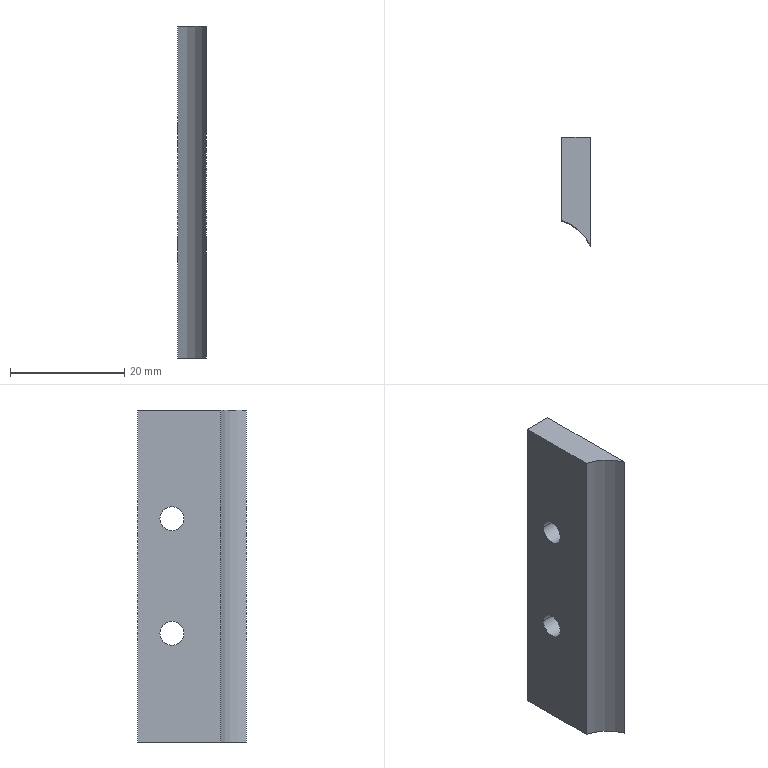Part | SolidWorks | features Extrusion 1, ICE 1 | 1 solid | 10 faces | box 5 x 19 x 58 mm | volume 4522 mm3 | cylinder 5 | plane 5 | commonest cylinder face diameters 4.2 x4 15.6 x1
STEP:
#1=CARTESIAN_POINT('',(2.222,2.186,19.));
#2=VERTEX_POINT('',#1);
#3=CARTESIAN_POINT('',(2.222,-2.014,19.));
#4=VERTEX_POINT('',#3);
#5=CARTESIAN_POINT('',(2.222,0.08586,19.));
#6=DIRECTION('',(-1.,0.,0.));
#7=DIRECTION('',(0.,-1.,0.));
#8=AXIS2_PLACEMENT_3D('',#5,#6,#7);
#9=CIRCLE('',#8,2.1);
#10=EDGE_CURVE('',#2,#4,#9,.T.);
#11=ORIENTED_EDGE('',*,*,#10,.F.);
#12=CARTESIAN_POINT('',(-2.778,2.186,19.));
#13=VERTEX_POINT('',#12);
#14=CARTESIAN_POINT('',(2.222,2.186,19.));
#15=DIRECTION('',(-1.,0.,0.));
#16=VECTOR('',#15,1000.);
#17=LINE('',#14,#16);
#18=EDGE_CURVE('',#2,#13,#17,.T.);
#19=ORIENTED_EDGE('',*,*,#18,.T.);
#20=CARTESIAN_POINT('',(-2.778,-2.014,19.));
#21=VERTEX_POINT('',#20);
#22=CARTESIAN_POINT('',(-2.778,0.08586,19.));
#23=DIRECTION('',(-1.,0.,0.));
#24=DIRECTION('',(0.,-1.,0.));
#25=AXIS2_PLACEMENT_3D('',#22,#23,#24);
#26=CIRCLE('',#25,2.1);
#27=EDGE_CURVE('',#13,#21,#26,.T.);
#28=ORIENTED_EDGE('',*,*,#27,.T.);
#29=CARTESIAN_POINT('',(2.222,-2.014,19.));
#30=DIRECTION('',(-1.,0.,0.));
#31=VECTOR('',#30,1000.);
#32=LINE('',#29,#31);
#33=EDGE_CURVE('',#4,#21,#32,.T.);
#34=ORIENTED_EDGE('',*,*,#33,.F.);
#35=EDGE_LOOP('',(#11,#19,#28,#34));
#36=FACE_OUTER_BOUND('',#35,.T.);
#37=CARTESIAN_POINT('',(2.222,0.08586,19.));
#38=DIRECTION('',(-1.,0.,0.));
#39=DIRECTION('',(0.,-1.,0.));
#40=AXIS2_PLACEMENT_3D('',#37,#38,#39);
#41=CYLINDRICAL_SURFACE('',#40,2.1);
#42=ADVANCED_FACE('',(#36),#41,.F.);
#43=CARTESIAN_POINT('',(2.222,2.186,39.));
#44=VERTEX_POINT('',#43);
#45=CARTESIAN_POINT('',(2.222,-2.014,39.));
#46=VERTEX_POINT('',#45);
#47=CARTESIAN_POINT('',(2.222,0.08586,39.));
#48=DIRECTION('',(-1.,0.,0.));
#49=DIRECTION('',(0.,-1.,0.));
#50=AXIS2_PLACEMENT_3D('',#47,#48,#49);
#51=CIRCLE('',#50,2.1);
#52=EDGE_CURVE('',#44,#46,#51,.T.);
#53=ORIENTED_EDGE('',*,*,#52,.F.);
#54=CARTESIAN_POINT('',(-2.778,2.186,39.));
#55=VERTEX_POINT('',#54);
#56=CARTESIAN_POINT('',(2.222,2.186,39.));
#57=DIRECTION('',(-1.,0.,0.));
#58=VECTOR('',#57,1000.);
#59=LINE('',#56,#58);
#60=EDGE_CURVE('',#44,#55,#59,.T.);
#61=ORIENTED_EDGE('',*,*,#60,.T.);
#62=CARTESIAN_POINT('',(-2.778,-2.014,39.));
#63=VERTEX_POINT('',#62);
#64=CARTESIAN_POINT('',(-2.778,0.08586,39.));
#65=DIRECTION('',(-1.,0.,0.));
#66=DIRECTION('',(0.,-1.,0.));
#67=AXIS2_PLACEMENT_3D('',#64,#65,#66);
#68=CIRCLE('',#67,2.1);
#69=EDGE_CURVE('',#55,#63,#68,.T.);
#70=ORIENTED_EDGE('',*,*,#69,.T.);
#71=CARTESIAN_POINT('',(2.222,-2.014,39.));
#72=DIRECTION('',(-1.,0.,0.));
#73=VECTOR('',#72,1000.);
#74=LINE('',#71,#73);
#75=EDGE_CURVE('',#46,#63,#74,.T.);
#76=ORIENTED_EDGE('',*,*,#75,.F.);
#77=EDGE_LOOP('',(#53,#61,#70,#76));
#78=FACE_OUTER_BOUND('',#77,.T.);
#79=CARTESIAN_POINT('',(2.222,0.08586,39.));
#80=DIRECTION('',(-1.,0.,0.));
#81=DIRECTION('',(0.,-1.,0.));
#82=AXIS2_PLACEMENT_3D('',#79,#80,#81);
#83=CYLINDRICAL_SURFACE('',#82,2.1);
#84=ADVANCED_FACE('',(#78),#83,.F.);
#85=CARTESIAN_POINT('',(-2.778,0.08586,19.));
#86=DIRECTION('',(-1.,0.,0.));
#87=DIRECTION('',(0.,-1.,0.));
#88=AXIS2_PLACEMENT_3D('',#85,#86,#87);
#89=CIRCLE('',#88,2.1);
#90=EDGE_CURVE('',#21,#13,#89,.T.);
#91=ORIENTED_EDGE('',*,*,#90,.F.);
#92=ORIENTED_EDGE('',*,*,#27,.F.);
#93=EDGE_LOOP('',(#91,#92));
#94=FACE_BOUND('',#93,.T.);
#95=CARTESIAN_POINT('',(-2.778,0.08586,39.));
#96=DIRECTION('',(-1.,0.,0.));
#97=DIRECTION('',(0.,-1.,0.));
#98=AXIS2_PLACEMENT_3D('',#95,#96,#97);
#99=CIRCLE('',#98,2.1);
#100=EDGE_CURVE('',#63,#55,#99,.T.);
#101=ORIENTED_EDGE('',*,*,#100,.F.);
#102=ORIENTED_EDGE('',*,*,#69,.F.);
#103=EDGE_LOOP('',(#101,#102));
#104=FACE_BOUND('',#103,.T.);
#105=CARTESIAN_POINT('',(-2.778,6.086,0.));
#106=VERTEX_POINT('',#105);
#107=CARTESIAN_POINT('',(-2.778,-8.431,0.));
#108=VERTEX_POINT('',#107);
#109=CARTESIAN_POINT('',(-2.778,6.086,0.));
#110=DIRECTION('',(0.,-1.,0.));
#111=VECTOR('',#110,1000.);
#112=LINE('',#109,#111);
#113=EDGE_CURVE('',#106,#108,#112,.T.);
#114=ORIENTED_EDGE('',*,*,#113,.T.);
#115=CARTESIAN_POINT('',(-2.778,-8.431,58.));
#116=VERTEX_POINT('',#115);
#117=CARTESIAN_POINT('',(-2.778,-8.431,58.));
#118=DIRECTION('',(0.,0.,-1.));
#119=VECTOR('',#118,1000.);
#120=LINE('',#117,#119);
#121=EDGE_CURVE('',#116,#108,#120,.T.);
#122=ORIENTED_EDGE('',*,*,#121,.F.);
#123=CARTESIAN_POINT('',(-2.778,6.086,58.));
#124=VERTEX_POINT('',#123);
#125=CARTESIAN_POINT('',(-2.778,6.086,58.));
#126=DIRECTION('',(0.,-1.,0.));
#127=VECTOR('',#126,1000.);
#128=LINE('',#125,#127);
#129=EDGE_CURVE('',#124,#116,#128,.T.);
#130=ORIENTED_EDGE('',*,*,#129,.F.);
#131=CARTESIAN_POINT('',(-2.778,6.086,58.));
#132=DIRECTION('',(0.,0.,-1.));
#133=VECTOR('',#132,1000.);
#134=LINE('',#131,#133);
#135=EDGE_CURVE('',#124,#106,#134,.T.);
#136=ORIENTED_EDGE('',*,*,#135,.T.);
#137=EDGE_LOOP('',(#114,#122,#130,#136));
#138=FACE_OUTER_BOUND('',#137,.T.);
#139=CARTESIAN_POINT('',(-2.778,6.086,58.));
#140=DIRECTION('',(1.,0.,0.));
#141=DIRECTION('',(0.,1.,0.));
#142=AXIS2_PLACEMENT_3D('',#139,#140,#141);
#143=PLANE('',#142);
#144=ADVANCED_FACE('',(#94,#104,#138),#143,.F.);
#145=CARTESIAN_POINT('',(2.222,-12.914,0.));
#146=VERTEX_POINT('',#145);
#147=CARTESIAN_POINT('',(-4.978,-15.914,0.));
#148=DIRECTION('',(0.,0.,-1.));
#149=DIRECTION('',(1.,0.,0.));
#150=AXIS2_PLACEMENT_3D('',#147,#148,#149);
#151=CIRCLE('',#150,7.8);
#152=EDGE_CURVE('',#108,#146,#151,.T.);
#153=ORIENTED_EDGE('',*,*,#152,.T.);
#154=CARTESIAN_POINT('',(2.222,-12.914,58.));
#155=VERTEX_POINT('',#154);
#156=CARTESIAN_POINT('',(2.222,-12.914,58.));
#157=DIRECTION('',(0.,0.,-1.));
#158=VECTOR('',#157,1000.);
#159=LINE('',#156,#158);
#160=EDGE_CURVE('',#155,#146,#159,.T.);
#161=ORIENTED_EDGE('',*,*,#160,.F.);
#162=CARTESIAN_POINT('',(-4.978,-15.914,58.));
#163=DIRECTION('',(0.,0.,-1.));
#164=DIRECTION('',(1.,0.,0.));
#165=AXIS2_PLACEMENT_3D('',#162,#163,#164);
#166=CIRCLE('',#165,7.8);
#167=EDGE_CURVE('',#116,#155,#166,.T.);
#168=ORIENTED_EDGE('',*,*,#167,.F.);
#169=ORIENTED_EDGE('',*,*,#121,.T.);
#170=EDGE_LOOP('',(#153,#161,#168,#169));
#171=FACE_OUTER_BOUND('',#170,.T.);
#172=CARTESIAN_POINT('',(-4.978,-15.914,58.));
#173=DIRECTION('',(0.,0.,-1.));
#174=DIRECTION('',(-1.,0.,0.));
#175=AXIS2_PLACEMENT_3D('',#172,#173,#174);
#176=CYLINDRICAL_SURFACE('',#175,7.8);
#177=ADVANCED_FACE('',(#171),#176,.F.);
#178=CARTESIAN_POINT('',(2.222,0.08586,19.));
#179=DIRECTION('',(-1.,0.,0.));
#180=DIRECTION('',(0.,-1.,0.));
#181=AXIS2_PLACEMENT_3D('',#178,#179,#180);
#182=CIRCLE('',#181,2.1);
#183=EDGE_CURVE('',#4,#2,#182,.T.);
#184=ORIENTED_EDGE('',*,*,#183,.T.);
#185=ORIENTED_EDGE('',*,*,#10,.T.);
#186=EDGE_LOOP('',(#184,#185));
#187=FACE_BOUND('',#186,.T.);
#188=CARTESIAN_POINT('',(2.222,0.08586,39.));
#189=DIRECTION('',(-1.,0.,0.));
#190=DIRECTION('',(0.,-1.,0.));
#191=AXIS2_PLACEMENT_3D('',#188,#189,#190);
#192=CIRCLE('',#191,2.1);
#193=EDGE_CURVE('',#46,#44,#192,.T.);
#194=ORIENTED_EDGE('',*,*,#193,.T.);
#195=ORIENTED_EDGE('',*,*,#52,.T.);
#196=EDGE_LOOP('',(#194,#195));
#197=FACE_BOUND('',#196,.T.);
#198=CARTESIAN_POINT('',(2.222,6.086,0.));
#199=VERTEX_POINT('',#198);
#200=CARTESIAN_POINT('',(2.222,6.086,0.));
#201=DIRECTION('',(0.,1.,0.));
#202=VECTOR('',#201,1000.);
#203=LINE('',#200,#202);
#204=EDGE_CURVE('',#146,#199,#203,.T.);
#205=ORIENTED_EDGE('',*,*,#204,.T.);
#206=CARTESIAN_POINT('',(2.222,6.086,58.));
#207=VERTEX_POINT('',#206);
#208=CARTESIAN_POINT('',(2.222,6.086,58.));
#209=DIRECTION('',(0.,0.,-1.));
#210=VECTOR('',#209,1000.);
#211=LINE('',#208,#210);
#212=EDGE_CURVE('',#207,#199,#211,.T.);
#213=ORIENTED_EDGE('',*,*,#212,.F.);
#214=CARTESIAN_POINT('',(2.222,6.086,58.));
#215=DIRECTION('',(0.,1.,0.));
#216=VECTOR('',#215,1000.);
#217=LINE('',#214,#216);
#218=EDGE_CURVE('',#155,#207,#217,.T.);
#219=ORIENTED_EDGE('',*,*,#218,.F.);
#220=ORIENTED_EDGE('',*,*,#160,.T.);
#221=EDGE_LOOP('',(#205,#213,#219,#220));
#222=FACE_OUTER_BOUND('',#221,.T.);
#223=CARTESIAN_POINT('',(2.222,6.086,58.));
#224=DIRECTION('',(-1.,0.,0.));
#225=DIRECTION('',(0.,-1.,0.));
#226=AXIS2_PLACEMENT_3D('',#223,#224,#225);
#227=PLANE('',#226);
#228=ADVANCED_FACE('',(#187,#197,#222),#227,.F.);
#229=CARTESIAN_POINT('',(-2.778,6.086,0.));
#230=DIRECTION('',(-1.,0.,0.));
#231=VECTOR('',#230,1000.);
#232=LINE('',#229,#231);
#233=EDGE_CURVE('',#199,#106,#232,.T.);
#234=ORIENTED_EDGE('',*,*,#233,.T.);
#235=ORIENTED_EDGE('',*,*,#135,.F.);
#236=CARTESIAN_POINT('',(-2.778,6.086,58.));
#237=DIRECTION('',(-1.,0.,0.));
#238=VECTOR('',#237,1000.);
#239=LINE('',#236,#238);
#240=EDGE_CURVE('',#207,#124,#239,.T.);
#241=ORIENTED_EDGE('',*,*,#240,.F.);
#242=ORIENTED_EDGE('',*,*,#212,.T.);
#243=EDGE_LOOP('',(#234,#235,#241,#242));
#244=FACE_OUTER_BOUND('',#243,.T.);
#245=CARTESIAN_POINT('',(-2.778,6.086,58.));
#246=DIRECTION('',(0.,-1.,0.));
#247=DIRECTION('',(0.,0.,-1.));
#248=AXIS2_PLACEMENT_3D('',#245,#246,#247);
#249=PLANE('',#248);
#250=ADVANCED_FACE('',(#244),#249,.F.);
#251=ORIENTED_EDGE('',*,*,#129,.T.);
#252=ORIENTED_EDGE('',*,*,#167,.T.);
#253=ORIENTED_EDGE('',*,*,#218,.T.);
#254=ORIENTED_EDGE('',*,*,#240,.T.);
#255=EDGE_LOOP('',(#251,#252,#253,#254));
#256=FACE_OUTER_BOUND('',#255,.T.);
#257=CARTESIAN_POINT('',(-4.978,-15.914,58.));
#258=DIRECTION('',(0.,0.,1.));
#259=DIRECTION('',(1.,0.,0.));
#260=AXIS2_PLACEMENT_3D('',#257,#258,#259);
#261=PLANE('',#260);
#262=ADVANCED_FACE('',(#256),#261,.T.);
#263=ORIENTED_EDGE('',*,*,#113,.F.);
#264=ORIENTED_EDGE('',*,*,#233,.F.);
#265=ORIENTED_EDGE('',*,*,#204,.F.);
#266=ORIENTED_EDGE('',*,*,#152,.F.);
#267=EDGE_LOOP('',(#263,#264,#265,#266));
#268=FACE_OUTER_BOUND('',#267,.T.);
#269=CARTESIAN_POINT('',(-4.978,-15.914,0.));
#270=DIRECTION('',(0.,0.,1.));
#271=DIRECTION('',(1.,0.,0.));
#272=AXIS2_PLACEMENT_3D('',#269,#270,#271);
#273=PLANE('',#272);
#274=ADVANCED_FACE('',(#268),#273,.F.);
#275=ORIENTED_EDGE('',*,*,#60,.F.);
#276=ORIENTED_EDGE('',*,*,#193,.F.);
#277=ORIENTED_EDGE('',*,*,#75,.T.);
#278=ORIENTED_EDGE('',*,*,#100,.T.);
#279=EDGE_LOOP('',(#275,#276,#277,#278));
#280=FACE_OUTER_BOUND('',#279,.T.);
#281=CARTESIAN_POINT('',(2.222,0.08586,39.));
#282=DIRECTION('',(-1.,0.,0.));
#283=DIRECTION('',(0.,-1.,0.));
#284=AXIS2_PLACEMENT_3D('',#281,#282,#283);
#285=CYLINDRICAL_SURFACE('',#284,2.1);
#286=ADVANCED_FACE('',(#280),#285,.F.);
#287=ORIENTED_EDGE('',*,*,#18,.F.);
#288=ORIENTED_EDGE('',*,*,#183,.F.);
#289=ORIENTED_EDGE('',*,*,#33,.T.);
#290=ORIENTED_EDGE('',*,*,#90,.T.);
#291=EDGE_LOOP('',(#287,#288,#289,#290));
#292=FACE_OUTER_BOUND('',#291,.T.);
#293=CARTESIAN_POINT('',(2.222,0.08586,19.));
#294=DIRECTION('',(-1.,0.,0.));
#295=DIRECTION('',(0.,-1.,0.));
#296=AXIS2_PLACEMENT_3D('',#293,#294,#295);
#297=CYLINDRICAL_SURFACE('',#296,2.1);
#298=ADVANCED_FACE('',(#292),#297,.F.);
#299=CLOSED_SHELL('',(#42,#84,#144,#177,#228,#250,#262,#274,#286,#298));
#300=MANIFOLD_SOLID_BREP('',#299);
#301=CARTESIAN_POINT('',(0.,0.,0.));
#302=DIRECTION('',(0.,0.,1.));
#303=DIRECTION('',(1.,0.,0.));
#304=AXIS2_PLACEMENT_3D('',#301,#302,#303);
#305=(LENGTH_UNIT()NAMED_UNIT(*)SI_UNIT(.MILLI.,.METRE.));
#306=UNCERTAINTY_MEASURE_WITH_UNIT(LENGTH_MEASURE(0.00001),#305,'','');
#307=(NAMED_UNIT(*)PLANE_ANGLE_UNIT()SI_UNIT($,.RADIAN.));
#308=(NAMED_UNIT(*)SI_UNIT($,.STERADIAN.)SOLID_ANGLE_UNIT());
#309=(GEOMETRIC_REPRESENTATION_CONTEXT(3)GLOBAL_UNCERTAINTY_ASSIGNED_CONTEXT((#306))GLOBAL_UNIT_ASSIGNED_CONTEXT((#305,#307,#308))REPRESENTATION_CONTEXT('',''));
#310=ADVANCED_BREP_SHAPE_REPRESENTATION('',(#300,#304),#309);